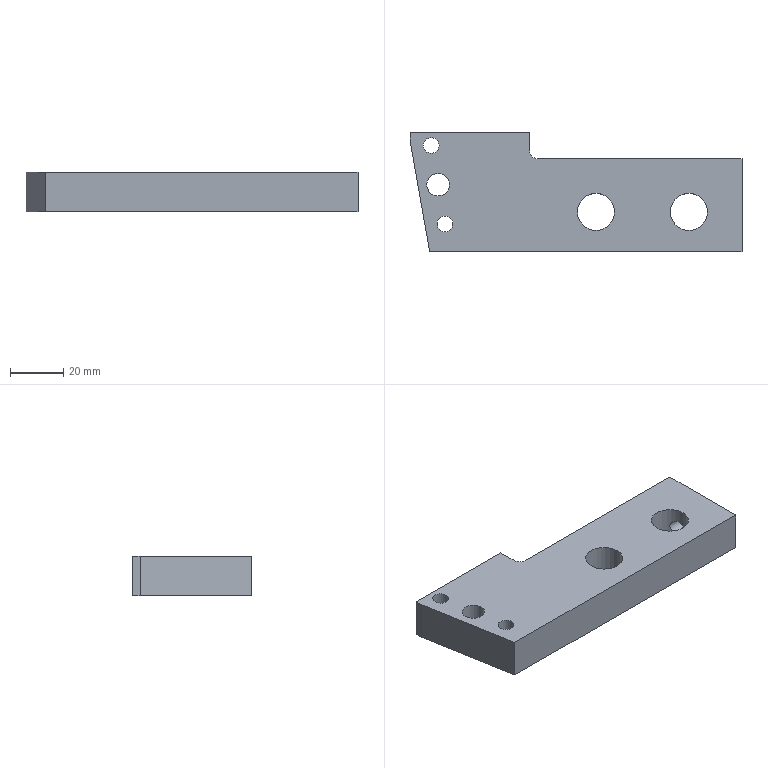Part | NX | features BREP 1 | 1 solid | 19 faces | box 125 x 45 x 15 mm | volume 63182 mm3 | plane 9 | cylinder 8 | cone 2 | commonest cylinder face diameters 6 x3 5 x2 14 x2 8.5 x1
STEP:
#1=CARTESIAN_POINT('',(62.5,-5.,-2.5));
#2=VERTEX_POINT('',#1);
#3=CARTESIAN_POINT('',(62.5,-5.,0.));
#4=DIRECTION('',(1.,0.,0.));
#5=DIRECTION('',(0.,0.,-1.));
#6=AXIS2_PLACEMENT_3D('',#3,#4,#5);
#7=CIRCLE('',#6,2.5);
#8=EDGE_CURVE('',#2,#2,#7,.T.);
#9=ORIENTED_EDGE('',*,*,#8,.F.);
#10=EDGE_LOOP('',(#9));
#11=FACE_BOUND('',#10,.T.);
#12=CARTESIAN_POINT('',(62.5,-22.5,-7.5));
#13=VERTEX_POINT('',#12);
#14=CARTESIAN_POINT('',(62.5,12.5,-7.5));
#15=VERTEX_POINT('',#14);
#16=CARTESIAN_POINT('',(62.5,-22.5,-7.5));
#17=DIRECTION('',(0.,1.,0.));
#18=VECTOR('',#17,1000.);
#19=LINE('',#16,#18);
#20=EDGE_CURVE('',#13,#15,#19,.T.);
#21=ORIENTED_EDGE('',*,*,#20,.T.);
#22=CARTESIAN_POINT('',(62.5,12.5,7.5));
#23=VERTEX_POINT('',#22);
#24=CARTESIAN_POINT('',(62.5,12.5,-88.123));
#25=DIRECTION('',(0.,0.,1.));
#26=VECTOR('',#25,1000.);
#27=LINE('',#24,#26);
#28=EDGE_CURVE('',#15,#23,#27,.T.);
#29=ORIENTED_EDGE('',*,*,#28,.T.);
#30=CARTESIAN_POINT('',(62.5,-22.5,7.5));
#31=VERTEX_POINT('',#30);
#32=CARTESIAN_POINT('',(62.5,-22.5,7.5));
#33=DIRECTION('',(0.,1.,0.));
#34=VECTOR('',#33,1000.);
#35=LINE('',#32,#34);
#36=EDGE_CURVE('',#31,#23,#35,.T.);
#37=ORIENTED_EDGE('',*,*,#36,.F.);
#38=CARTESIAN_POINT('',(62.5,-22.5,7.5));
#39=DIRECTION('',(0.,0.,-1.));
#40=VECTOR('',#39,1000.);
#41=LINE('',#38,#40);
#42=EDGE_CURVE('',#31,#13,#41,.T.);
#43=ORIENTED_EDGE('',*,*,#42,.T.);
#44=EDGE_LOOP('',(#21,#29,#37,#43));
#45=FACE_BOUND('',#44,.T.);
#46=CARTESIAN_POINT('',(62.5,-22.5,7.5));
#47=DIRECTION('',(-1.,0.,0.));
#48=DIRECTION('',(0.,0.,-1.));
#49=AXIS2_PLACEMENT_3D('',#46,#47,#48);
#50=PLANE('',#49);
#51=ADVANCED_FACE('',(#11,#45),#50,.F.);
#52=CARTESIAN_POINT('',(-17.5,22.5,7.5));
#53=VERTEX_POINT('',#52);
#54=CARTESIAN_POINT('',(-62.5,22.5,7.5));
#55=VERTEX_POINT('',#54);
#56=CARTESIAN_POINT('',(-62.5,22.5,7.5));
#57=DIRECTION('',(-1.,0.,0.));
#58=VECTOR('',#57,1000.);
#59=LINE('',#56,#58);
#60=EDGE_CURVE('',#53,#55,#59,.T.);
#61=ORIENTED_EDGE('',*,*,#60,.F.);
#62=CARTESIAN_POINT('',(-17.5,22.5,-7.5));
#63=VERTEX_POINT('',#62);
#64=CARTESIAN_POINT('',(-17.5,22.5,-88.123));
#65=DIRECTION('',(0.,0.,1.));
#66=VECTOR('',#65,1000.);
#67=LINE('',#64,#66);
#68=EDGE_CURVE('',#63,#53,#67,.T.);
#69=ORIENTED_EDGE('',*,*,#68,.F.);
#70=CARTESIAN_POINT('',(-62.5,22.5,-7.5));
#71=VERTEX_POINT('',#70);
#72=CARTESIAN_POINT('',(-62.5,22.5,-7.5));
#73=DIRECTION('',(-1.,0.,0.));
#74=VECTOR('',#73,1000.);
#75=LINE('',#72,#74);
#76=EDGE_CURVE('',#63,#71,#75,.T.);
#77=ORIENTED_EDGE('',*,*,#76,.T.);
#78=CARTESIAN_POINT('',(-62.5,22.5,7.5));
#79=DIRECTION('',(0.,0.,-1.));
#80=VECTOR('',#79,1000.);
#81=LINE('',#78,#80);
#82=EDGE_CURVE('',#55,#71,#81,.T.);
#83=ORIENTED_EDGE('',*,*,#82,.F.);
#84=EDGE_LOOP('',(#61,#69,#77,#83));
#85=FACE_BOUND('',#84,.T.);
#86=CARTESIAN_POINT('',(-62.5,22.5,7.5));
#87=DIRECTION('',(0.,-1.,0.));
#88=DIRECTION('',(0.,0.,1.));
#89=AXIS2_PLACEMENT_3D('',#86,#87,#88);
#90=PLANE('',#89);
#91=ADVANCED_FACE('',(#85),#90,.F.);
#92=CARTESIAN_POINT('',(-62.5,19.5,-7.5));
#93=VERTEX_POINT('',#92);
#94=CARTESIAN_POINT('',(-62.5,-22.5,-7.5));
#95=DIRECTION('',(0.,-1.,0.));
#96=VECTOR('',#95,1000.);
#97=LINE('',#94,#96);
#98=EDGE_CURVE('',#71,#93,#97,.T.);
#99=ORIENTED_EDGE('',*,*,#98,.T.);
#100=CARTESIAN_POINT('',(-62.5,19.5,7.5));
#101=VERTEX_POINT('',#100);
#102=CARTESIAN_POINT('',(-62.5,19.5,-50.148));
#103=DIRECTION('',(0.,0.,1.));
#104=VECTOR('',#103,1000.);
#105=LINE('',#102,#104);
#106=EDGE_CURVE('',#93,#101,#105,.T.);
#107=ORIENTED_EDGE('',*,*,#106,.T.);
#108=CARTESIAN_POINT('',(-62.5,-22.5,7.5));
#109=DIRECTION('',(0.,-1.,0.));
#110=VECTOR('',#109,1000.);
#111=LINE('',#108,#110);
#112=EDGE_CURVE('',#55,#101,#111,.T.);
#113=ORIENTED_EDGE('',*,*,#112,.F.);
#114=ORIENTED_EDGE('',*,*,#82,.T.);
#115=EDGE_LOOP('',(#99,#107,#113,#114));
#116=FACE_BOUND('',#115,.T.);
#117=CARTESIAN_POINT('',(-62.5,-22.5,7.5));
#118=DIRECTION('',(1.,0.,0.));
#119=DIRECTION('',(0.,0.,1.));
#120=AXIS2_PLACEMENT_3D('',#117,#118,#119);
#121=PLANE('',#120);
#122=ADVANCED_FACE('',(#116),#121,.F.);
#123=CARTESIAN_POINT('',(-55.094,-22.5,7.5));
#124=VERTEX_POINT('',#123);
#125=CARTESIAN_POINT('',(-62.5,-22.5,7.5));
#126=DIRECTION('',(1.,0.,0.));
#127=VECTOR('',#126,1000.);
#128=LINE('',#125,#127);
#129=EDGE_CURVE('',#124,#31,#128,.T.);
#130=ORIENTED_EDGE('',*,*,#129,.F.);
#131=CARTESIAN_POINT('',(-55.094,-22.5,-7.5));
#132=VERTEX_POINT('',#131);
#133=CARTESIAN_POINT('',(-55.094,-22.5,-50.148));
#134=DIRECTION('',(0.,0.,1.));
#135=VECTOR('',#134,1000.);
#136=LINE('',#133,#135);
#137=EDGE_CURVE('',#132,#124,#136,.T.);
#138=ORIENTED_EDGE('',*,*,#137,.F.);
#139=CARTESIAN_POINT('',(-62.5,-22.5,-7.5));
#140=DIRECTION('',(1.,0.,0.));
#141=VECTOR('',#140,1000.);
#142=LINE('',#139,#141);
#143=EDGE_CURVE('',#132,#13,#142,.T.);
#144=ORIENTED_EDGE('',*,*,#143,.T.);
#145=ORIENTED_EDGE('',*,*,#42,.F.);
#146=EDGE_LOOP('',(#130,#138,#144,#145));
#147=FACE_BOUND('',#146,.T.);
#148=CARTESIAN_POINT('',(-62.5,-22.5,7.5));
#149=DIRECTION('',(0.,1.,0.));
#150=DIRECTION('',(0.,0.,-1.));
#151=AXIS2_PLACEMENT_3D('',#148,#149,#150);
#152=PLANE('',#151);
#153=ADVANCED_FACE('',(#147),#152,.F.);
#154=CARTESIAN_POINT('',(49.5,-7.5,7.5));
#155=VERTEX_POINT('',#154);
#156=CARTESIAN_POINT('',(42.5,-7.5,7.5));
#157=DIRECTION('',(0.,0.,1.));
#158=DIRECTION('',(1.,0.,0.));
#159=AXIS2_PLACEMENT_3D('',#156,#157,#158);
#160=CIRCLE('',#159,7.);
#161=EDGE_CURVE('',#155,#155,#160,.T.);
#162=ORIENTED_EDGE('',*,*,#161,.F.);
#163=EDGE_LOOP('',(#162));
#164=FACE_BOUND('',#163,.T.);
#165=CARTESIAN_POINT('',(14.5,-7.5,7.5));
#166=VERTEX_POINT('',#165);
#167=CARTESIAN_POINT('',(7.5,-7.5,7.5));
#168=DIRECTION('',(0.,0.,1.));
#169=DIRECTION('',(1.,0.,0.));
#170=AXIS2_PLACEMENT_3D('',#167,#168,#169);
#171=CIRCLE('',#170,7.);
#172=EDGE_CURVE('',#166,#166,#171,.T.);
#173=ORIENTED_EDGE('',*,*,#172,.F.);
#174=EDGE_LOOP('',(#173));
#175=FACE_BOUND('',#174,.T.);
#176=CARTESIAN_POINT('',(-47.677,2.728,7.5));
#177=VERTEX_POINT('',#176);
#178=CARTESIAN_POINT('',(-51.927,2.728,7.5));
#179=DIRECTION('',(0.,0.,1.));
#180=DIRECTION('',(1.,0.,0.));
#181=AXIS2_PLACEMENT_3D('',#178,#179,#180);
#182=CIRCLE('',#181,4.25);
#183=EDGE_CURVE('',#177,#177,#182,.T.);
#184=ORIENTED_EDGE('',*,*,#183,.F.);
#185=EDGE_LOOP('',(#184));
#186=FACE_BOUND('',#185,.T.);
#187=CARTESIAN_POINT('',(-51.532,17.5,7.5));
#188=VERTEX_POINT('',#187);
#189=CARTESIAN_POINT('',(-54.532,17.5,7.5));
#190=DIRECTION('',(0.,0.,1.));
#191=DIRECTION('',(1.,0.,0.));
#192=AXIS2_PLACEMENT_3D('',#189,#190,#191);
#193=CIRCLE('',#192,3.);
#194=EDGE_CURVE('',#188,#188,#193,.T.);
#195=ORIENTED_EDGE('',*,*,#194,.F.);
#196=EDGE_LOOP('',(#195));
#197=FACE_BOUND('',#196,.T.);
#198=CARTESIAN_POINT('',(-46.322,-12.044,7.5));
#199=VERTEX_POINT('',#198);
#200=CARTESIAN_POINT('',(-49.322,-12.044,7.5));
#201=DIRECTION('',(0.,0.,1.));
#202=DIRECTION('',(1.,0.,0.));
#203=AXIS2_PLACEMENT_3D('',#200,#201,#202);
#204=CIRCLE('',#203,3.);
#205=EDGE_CURVE('',#199,#199,#204,.T.);
#206=ORIENTED_EDGE('',*,*,#205,.F.);
#207=EDGE_LOOP('',(#206));
#208=FACE_BOUND('',#207,.T.);
#209=CARTESIAN_POINT('',(-14.5,12.5,7.5));
#210=VERTEX_POINT('',#209);
#211=CARTESIAN_POINT('',(62.5,12.5,7.5));
#212=DIRECTION('',(1.,0.,0.));
#213=VECTOR('',#212,1000.);
#214=LINE('',#211,#213);
#215=EDGE_CURVE('',#210,#23,#214,.T.);
#216=ORIENTED_EDGE('',*,*,#215,.F.);
#217=CARTESIAN_POINT('',(-17.5,15.5,7.5));
#218=VERTEX_POINT('',#217);
#219=CARTESIAN_POINT('',(-14.5,15.5,7.5));
#220=DIRECTION('',(0.,0.,-1.));
#221=DIRECTION('',(-1.,0.,0.));
#222=AXIS2_PLACEMENT_3D('',#219,#220,#221);
#223=CIRCLE('',#222,3.);
#224=EDGE_CURVE('',#210,#218,#223,.T.);
#225=ORIENTED_EDGE('',*,*,#224,.T.);
#226=CARTESIAN_POINT('',(-17.5,12.5,7.5));
#227=DIRECTION('',(0.,-1.,0.));
#228=VECTOR('',#227,1000.);
#229=LINE('',#226,#228);
#230=EDGE_CURVE('',#53,#218,#229,.T.);
#231=ORIENTED_EDGE('',*,*,#230,.F.);
#232=ORIENTED_EDGE('',*,*,#60,.T.);
#233=ORIENTED_EDGE('',*,*,#112,.T.);
#234=CARTESIAN_POINT('',(-62.5,19.5,7.5));
#235=DIRECTION('',(-0.1736,0.9848,0.));
#236=VECTOR('',#235,1000.);
#237=LINE('',#234,#236);
#238=EDGE_CURVE('',#124,#101,#237,.T.);
#239=ORIENTED_EDGE('',*,*,#238,.F.);
#240=ORIENTED_EDGE('',*,*,#129,.T.);
#241=ORIENTED_EDGE('',*,*,#36,.T.);
#242=EDGE_LOOP('',(#216,#225,#231,#232,#233,#239,#240,#241));
#243=FACE_BOUND('',#242,.T.);
#244=CARTESIAN_POINT('',(0.,0.,7.5));
#245=DIRECTION('',(0.,0.,-1.));
#246=DIRECTION('',(1.,0.,0.));
#247=AXIS2_PLACEMENT_3D('',#244,#245,#246);
#248=PLANE('',#247);
#249=ADVANCED_FACE('',(#164,#175,#186,#197,#208,#243),#248,.F.);
#250=CARTESIAN_POINT('',(49.5,-7.5,-7.5));
#251=VERTEX_POINT('',#250);
#252=CARTESIAN_POINT('',(42.5,-7.5,-7.5));
#253=DIRECTION('',(0.,0.,1.));
#254=DIRECTION('',(1.,0.,0.));
#255=AXIS2_PLACEMENT_3D('',#252,#253,#254);
#256=CIRCLE('',#255,7.);
#257=EDGE_CURVE('',#251,#251,#256,.T.);
#258=ORIENTED_EDGE('',*,*,#257,.T.);
#259=EDGE_LOOP('',(#258));
#260=FACE_BOUND('',#259,.T.);
#261=CARTESIAN_POINT('',(14.5,-7.5,-7.5));
#262=VERTEX_POINT('',#261);
#263=CARTESIAN_POINT('',(7.5,-7.5,-7.5));
#264=DIRECTION('',(0.,0.,1.));
#265=DIRECTION('',(1.,0.,0.));
#266=AXIS2_PLACEMENT_3D('',#263,#264,#265);
#267=CIRCLE('',#266,7.);
#268=EDGE_CURVE('',#262,#262,#267,.T.);
#269=ORIENTED_EDGE('',*,*,#268,.T.);
#270=EDGE_LOOP('',(#269));
#271=FACE_BOUND('',#270,.T.);
#272=CARTESIAN_POINT('',(-17.5,15.5,-7.5));
#273=VERTEX_POINT('',#272);
#274=CARTESIAN_POINT('',(-17.5,12.5,-7.5));
#275=DIRECTION('',(0.,-1.,0.));
#276=VECTOR('',#275,1000.);
#277=LINE('',#274,#276);
#278=EDGE_CURVE('',#63,#273,#277,.T.);
#279=ORIENTED_EDGE('',*,*,#278,.T.);
#280=CARTESIAN_POINT('',(-14.5,12.5,-7.5));
#281=VERTEX_POINT('',#280);
#282=CARTESIAN_POINT('',(-14.5,15.5,-7.5));
#283=DIRECTION('',(0.,0.,1.));
#284=DIRECTION('',(-1.,0.,0.));
#285=AXIS2_PLACEMENT_3D('',#282,#283,#284);
#286=CIRCLE('',#285,3.);
#287=EDGE_CURVE('',#273,#281,#286,.T.);
#288=ORIENTED_EDGE('',*,*,#287,.T.);
#289=CARTESIAN_POINT('',(62.5,12.5,-7.5));
#290=DIRECTION('',(1.,0.,0.));
#291=VECTOR('',#290,1000.);
#292=LINE('',#289,#291);
#293=EDGE_CURVE('',#281,#15,#292,.T.);
#294=ORIENTED_EDGE('',*,*,#293,.T.);
#295=ORIENTED_EDGE('',*,*,#20,.F.);
#296=ORIENTED_EDGE('',*,*,#143,.F.);
#297=CARTESIAN_POINT('',(-62.5,19.5,-7.5));
#298=DIRECTION('',(-0.1736,0.9848,0.));
#299=VECTOR('',#298,1000.);
#300=LINE('',#297,#299);
#301=EDGE_CURVE('',#132,#93,#300,.T.);
#302=ORIENTED_EDGE('',*,*,#301,.T.);
#303=ORIENTED_EDGE('',*,*,#98,.F.);
#304=ORIENTED_EDGE('',*,*,#76,.F.);
#305=EDGE_LOOP('',(#279,#288,#294,#295,#296,#302,#303,#304));
#306=FACE_BOUND('',#305,.T.);
#307=CARTESIAN_POINT('',(-47.677,2.728,-7.5));
#308=VERTEX_POINT('',#307);
#309=CARTESIAN_POINT('',(-51.927,2.728,-7.5));
#310=DIRECTION('',(0.,0.,1.));
#311=DIRECTION('',(1.,0.,0.));
#312=AXIS2_PLACEMENT_3D('',#309,#310,#311);
#313=CIRCLE('',#312,4.25);
#314=EDGE_CURVE('',#308,#308,#313,.T.);
#315=ORIENTED_EDGE('',*,*,#314,.T.);
#316=EDGE_LOOP('',(#315));
#317=FACE_BOUND('',#316,.T.);
#318=CARTESIAN_POINT('',(-51.532,17.5,-7.5));
#319=VERTEX_POINT('',#318);
#320=CARTESIAN_POINT('',(-54.532,17.5,-7.5));
#321=DIRECTION('',(0.,0.,1.));
#322=DIRECTION('',(1.,0.,0.));
#323=AXIS2_PLACEMENT_3D('',#320,#321,#322);
#324=CIRCLE('',#323,3.);
#325=EDGE_CURVE('',#319,#319,#324,.T.);
#326=ORIENTED_EDGE('',*,*,#325,.T.);
#327=EDGE_LOOP('',(#326));
#328=FACE_BOUND('',#327,.T.);
#329=CARTESIAN_POINT('',(-46.322,-12.044,-7.5));
#330=VERTEX_POINT('',#329);
#331=CARTESIAN_POINT('',(-49.322,-12.044,-7.5));
#332=DIRECTION('',(0.,0.,1.));
#333=DIRECTION('',(1.,0.,0.));
#334=AXIS2_PLACEMENT_3D('',#331,#332,#333);
#335=CIRCLE('',#334,3.);
#336=EDGE_CURVE('',#330,#330,#335,.T.);
#337=ORIENTED_EDGE('',*,*,#336,.T.);
#338=EDGE_LOOP('',(#337));
#339=FACE_BOUND('',#338,.T.);
#340=CARTESIAN_POINT('',(0.,0.,-7.5));
#341=DIRECTION('',(0.,0.,-1.));
#342=DIRECTION('',(1.,0.,0.));
#343=AXIS2_PLACEMENT_3D('',#340,#341,#342);
#344=PLANE('',#343);
#345=ADVANCED_FACE('',(#260,#271,#306,#317,#328,#339),#344,.T.);
#346=ORIENTED_EDGE('',*,*,#137,.T.);
#347=ORIENTED_EDGE('',*,*,#238,.T.);
#348=ORIENTED_EDGE('',*,*,#106,.F.);
#349=ORIENTED_EDGE('',*,*,#301,.F.);
#350=EDGE_LOOP('',(#346,#347,#348,#349));
#351=FACE_BOUND('',#350,.T.);
#352=CARTESIAN_POINT('',(-62.5,19.5,-50.148));
#353=DIRECTION('',(0.9848,0.1736,0.));
#354=DIRECTION('',(0.1736,-0.9848,0.));
#355=AXIS2_PLACEMENT_3D('',#352,#353,#354);
#356=PLANE('',#355);
#357=ADVANCED_FACE('',(#351),#356,.F.);
#358=ORIENTED_EDGE('',*,*,#336,.F.);
#359=EDGE_LOOP('',(#358));
#360=FACE_BOUND('',#359,.T.);
#361=ORIENTED_EDGE('',*,*,#205,.T.);
#362=EDGE_LOOP('',(#361));
#363=FACE_BOUND('',#362,.T.);
#364=CARTESIAN_POINT('',(-49.322,-12.044,7.5));
#365=DIRECTION('',(0.,0.,1.));
#366=DIRECTION('',(-1.,0.,0.));
#367=AXIS2_PLACEMENT_3D('',#364,#365,#366);
#368=CYLINDRICAL_SURFACE('',#367,3.);
#369=ADVANCED_FACE('',(#360,#363),#368,.F.);
#370=ORIENTED_EDGE('',*,*,#325,.F.);
#371=EDGE_LOOP('',(#370));
#372=FACE_BOUND('',#371,.T.);
#373=ORIENTED_EDGE('',*,*,#194,.T.);
#374=EDGE_LOOP('',(#373));
#375=FACE_BOUND('',#374,.T.);
#376=CARTESIAN_POINT('',(-54.532,17.5,7.5));
#377=DIRECTION('',(0.,0.,1.));
#378=DIRECTION('',(-1.,0.,0.));
#379=AXIS2_PLACEMENT_3D('',#376,#377,#378);
#380=CYLINDRICAL_SURFACE('',#379,3.);
#381=ADVANCED_FACE('',(#372,#375),#380,.F.);
#382=ORIENTED_EDGE('',*,*,#314,.F.);
#383=EDGE_LOOP('',(#382));
#384=FACE_BOUND('',#383,.T.);
#385=ORIENTED_EDGE('',*,*,#183,.T.);
#386=EDGE_LOOP('',(#385));
#387=FACE_BOUND('',#386,.T.);
#388=CARTESIAN_POINT('',(-51.927,2.728,7.5));
#389=DIRECTION('',(0.,0.,1.));
#390=DIRECTION('',(-1.,0.,0.));
#391=AXIS2_PLACEMENT_3D('',#388,#389,#390);
#392=CYLINDRICAL_SURFACE('',#391,4.25);
#393=ADVANCED_FACE('',(#384,#387),#392,.F.);
#394=ORIENTED_EDGE('',*,*,#230,.T.);
#395=CARTESIAN_POINT('',(-17.5,15.5,-7.5));
#396=DIRECTION('',(0.,0.,-1.));
#397=VECTOR('',#396,1000.);
#398=LINE('',#395,#397);
#399=EDGE_CURVE('',#218,#273,#398,.T.);
#400=ORIENTED_EDGE('',*,*,#399,.T.);
#401=ORIENTED_EDGE('',*,*,#278,.F.);
#402=ORIENTED_EDGE('',*,*,#68,.T.);
#403=EDGE_LOOP('',(#394,#400,#401,#402));
#404=FACE_BOUND('',#403,.T.);
#405=CARTESIAN_POINT('',(-17.5,12.5,-88.123));
#406=DIRECTION('',(-1.,0.,0.));
#407=DIRECTION('',(0.,0.,-1.));
#408=AXIS2_PLACEMENT_3D('',#405,#406,#407);
#409=PLANE('',#408);
#410=ADVANCED_FACE('',(#404),#409,.F.);
#411=CARTESIAN_POINT('',(17.5,12.5,2.5));
#412=VERTEX_POINT('',#411);
#413=CARTESIAN_POINT('',(17.5,12.5,0.));
#414=DIRECTION('',(0.,1.,0.));
#415=DIRECTION('',(0.,0.,1.));
#416=AXIS2_PLACEMENT_3D('',#413,#414,#415);
#417=CIRCLE('',#416,2.5);
#418=EDGE_CURVE('',#412,#412,#417,.T.);
#419=ORIENTED_EDGE('',*,*,#418,.F.);
#420=EDGE_LOOP('',(#419));
#421=FACE_BOUND('',#420,.T.);
#422=ORIENTED_EDGE('',*,*,#293,.F.);
#423=CARTESIAN_POINT('',(-14.5,12.5,7.5));
#424=DIRECTION('',(0.,0.,1.));
#425=VECTOR('',#424,1000.);
#426=LINE('',#423,#425);
#427=EDGE_CURVE('',#281,#210,#426,.T.);
#428=ORIENTED_EDGE('',*,*,#427,.T.);
#429=ORIENTED_EDGE('',*,*,#215,.T.);
#430=ORIENTED_EDGE('',*,*,#28,.F.);
#431=EDGE_LOOP('',(#422,#428,#429,#430));
#432=FACE_BOUND('',#431,.T.);
#433=CARTESIAN_POINT('',(62.5,12.5,-88.123));
#434=DIRECTION('',(0.,-1.,0.));
#435=DIRECTION('',(-1.,0.,0.));
#436=AXIS2_PLACEMENT_3D('',#433,#434,#435);
#437=PLANE('',#436);
#438=ADVANCED_FACE('',(#421,#432),#437,.F.);
#439=ORIENTED_EDGE('',*,*,#268,.F.);
#440=EDGE_LOOP('',(#439));
#441=FACE_BOUND('',#440,.T.);
#442=ORIENTED_EDGE('',*,*,#172,.T.);
#443=EDGE_LOOP('',(#442));
#444=FACE_BOUND('',#443,.T.);
#445=CARTESIAN_POINT('',(7.5,-7.5,7.5));
#446=DIRECTION('',(0.,0.,1.));
#447=DIRECTION('',(-1.,0.,0.));
#448=AXIS2_PLACEMENT_3D('',#445,#446,#447);
#449=CYLINDRICAL_SURFACE('',#448,7.);
#450=ADVANCED_FACE('',(#441,#444),#449,.F.);
#451=CARTESIAN_POINT('',(47.5,-2.601,-0.7035));
#452=VERTEX_POINT('',#451);
#453=CARTESIAN_POINT('',(47.5,-2.601,0.7035));
#454=VERTEX_POINT('',#453);
#455=CARTESIAN_POINT('',(47.5,-2.601,-0.7035));
#456=CARTESIAN_POINT('',(47.45,-2.55,-0.2345));
#457=CARTESIAN_POINT('',(47.45,-2.55,0.2345));
#458=CARTESIAN_POINT('',(47.5,-2.601,0.7035));
#459=B_SPLINE_CURVE_WITH_KNOTS('',3,(#455,#456,#457,#458),.UNSPECIFIED.,.F.,.F.,(4,4),(0.,0.001407),.UNSPECIFIED.);
#460=EDGE_CURVE('',#452,#454,#459,.T.);
#461=ORIENTED_EDGE('',*,*,#460,.T.);
#462=CARTESIAN_POINT('',(47.5,-2.601,0.7035));
#463=CARTESIAN_POINT('',(47.669,-2.774,1.292));
#464=CARTESIAN_POINT('',(48.313,-3.475,2.198));
#465=CARTESIAN_POINT('',(49.199,-5.161,2.716));
#466=CARTESIAN_POINT('',(49.528,-6.996,1.898));
#467=CARTESIAN_POINT('',(49.486,-7.75,0.005277));
#468=CARTESIAN_POINT('',(49.528,-7.006,-1.885));
#469=CARTESIAN_POINT('',(49.205,-5.176,-2.717));
#470=CARTESIAN_POINT('',(48.312,-3.472,-2.199));
#471=CARTESIAN_POINT('',(47.669,-2.774,-1.293));
#472=CARTESIAN_POINT('',(47.5,-2.601,-0.7035));
#473=B_SPLINE_CURVE_WITH_KNOTS('',3,(#462,#463,#464,#465,#466,#467,#468,#469,#470,#471,#472),.UNSPECIFIED.,.F.,.F.,(4,1,1,1,1,1,1,1,4),(0.,0.001875,0.003749,0.005624,0.007499,0.009373,0.01125,0.01312,0.015),.UNSPECIFIED.);
#474=EDGE_CURVE('',#454,#452,#473,.T.);
#475=ORIENTED_EDGE('',*,*,#474,.T.);
#476=EDGE_LOOP('',(#461,#475));
#477=FACE_BOUND('',#476,.T.);
#478=ORIENTED_EDGE('',*,*,#257,.F.);
#479=EDGE_LOOP('',(#478));
#480=FACE_BOUND('',#479,.T.);
#481=ORIENTED_EDGE('',*,*,#161,.T.);
#482=EDGE_LOOP('',(#481));
#483=FACE_BOUND('',#482,.T.);
#484=CARTESIAN_POINT('',(42.5,-7.5,7.5));
#485=DIRECTION('',(0.,0.,1.));
#486=DIRECTION('',(-1.,0.,0.));
#487=AXIS2_PLACEMENT_3D('',#484,#485,#486);
#488=CYLINDRICAL_SURFACE('',#487,7.);
#489=ADVANCED_FACE('',(#477,#480,#483),#488,.F.);
#490=ORIENTED_EDGE('',*,*,#8,.T.);
#491=EDGE_LOOP('',(#490));
#492=FACE_BOUND('',#491,.T.);
#493=CARTESIAN_POINT('',(47.5,-5.,0.));
#494=DIRECTION('',(1.,0.,0.));
#495=DIRECTION('',(0.,0.,-1.));
#496=AXIS2_PLACEMENT_3D('',#493,#494,#495);
#497=CIRCLE('',#496,2.5);
#498=EDGE_CURVE('',#452,#454,#497,.T.);
#499=ORIENTED_EDGE('',*,*,#498,.F.);
#500=ORIENTED_EDGE('',*,*,#474,.F.);
#501=EDGE_LOOP('',(#499,#500));
#502=FACE_BOUND('',#501,.T.);
#503=CARTESIAN_POINT('',(62.5,-5.,0.));
#504=DIRECTION('',(1.,0.,0.));
#505=DIRECTION('',(0.,0.,1.));
#506=AXIS2_PLACEMENT_3D('',#503,#504,#505);
#507=CYLINDRICAL_SURFACE('',#506,2.5);
#508=ADVANCED_FACE('',(#492,#502),#507,.F.);
#509=ORIENTED_EDGE('',*,*,#498,.T.);
#510=ORIENTED_EDGE('',*,*,#460,.F.);
#511=EDGE_LOOP('',(#509,#510));
#512=FACE_BOUND('',#511,.T.);
#513=CARTESIAN_POINT('',(47.5,-5.,0.));
#514=DIRECTION('',(1.,0.,0.));
#515=DIRECTION('',(0.,0.,1.));
#516=AXIS2_PLACEMENT_3D('',#513,#514,#515);
#517=CONICAL_SURFACE('',#516,2.5,1.03);
#518=ADVANCED_FACE('',(#512),#517,.F.);
#519=CARTESIAN_POINT('',(17.5,-4.002,0.));
#520=VERTEX_POINT('',#519);
#521=VERTEX_LOOP('',#520);
#522=FACE_BOUND('',#521,.T.);
#523=CARTESIAN_POINT('',(17.5,-2.5,2.5));
#524=VERTEX_POINT('',#523);
#525=CARTESIAN_POINT('',(17.5,-2.5,0.));
#526=DIRECTION('',(0.,1.,0.));
#527=DIRECTION('',(0.,0.,1.));
#528=AXIS2_PLACEMENT_3D('',#525,#526,#527);
#529=CIRCLE('',#528,2.5);
#530=EDGE_CURVE('',#524,#524,#529,.T.);
#531=ORIENTED_EDGE('',*,*,#530,.T.);
#532=EDGE_LOOP('',(#531));
#533=FACE_BOUND('',#532,.T.);
#534=CARTESIAN_POINT('',(17.5,-2.5,0.));
#535=DIRECTION('',(0.,1.,0.));
#536=DIRECTION('',(0.,0.,-1.));
#537=AXIS2_PLACEMENT_3D('',#534,#535,#536);
#538=CONICAL_SURFACE('',#537,2.5,1.03);
#539=ADVANCED_FACE('',(#522,#533),#538,.F.);
#540=ORIENTED_EDGE('',*,*,#530,.F.);
#541=EDGE_LOOP('',(#540));
#542=FACE_BOUND('',#541,.T.);
#543=ORIENTED_EDGE('',*,*,#418,.T.);
#544=EDGE_LOOP('',(#543));
#545=FACE_BOUND('',#544,.T.);
#546=CARTESIAN_POINT('',(17.5,12.5,0.));
#547=DIRECTION('',(0.,1.,0.));
#548=DIRECTION('',(0.,0.,-1.));
#549=AXIS2_PLACEMENT_3D('',#546,#547,#548);
#550=CYLINDRICAL_SURFACE('',#549,2.5);
#551=ADVANCED_FACE('',(#542,#545),#550,.F.);
#552=ORIENTED_EDGE('',*,*,#287,.F.);
#553=ORIENTED_EDGE('',*,*,#399,.F.);
#554=ORIENTED_EDGE('',*,*,#224,.F.);
#555=ORIENTED_EDGE('',*,*,#427,.F.);
#556=EDGE_LOOP('',(#552,#553,#554,#555));
#557=FACE_BOUND('',#556,.T.);
#558=CARTESIAN_POINT('',(-14.5,15.5,-88.123));
#559=DIRECTION('',(0.,0.,-1.));
#560=DIRECTION('',(1.,0.,0.));
#561=AXIS2_PLACEMENT_3D('',#558,#559,#560);
#562=CYLINDRICAL_SURFACE('',#561,3.);
#563=ADVANCED_FACE('',(#557),#562,.F.);
#564=CLOSED_SHELL('',(#51,#91,#122,#153,#249,#345,#357,#369,#381,#393,#410,#438,#450,#489,#508,#518,#539,#551,#563));
#565=MANIFOLD_SOLID_BREP('',#564);
#566=(LENGTH_UNIT()NAMED_UNIT(*)SI_UNIT(.MILLI.,.METRE.));
#567=UNCERTAINTY_MEASURE_WITH_UNIT(LENGTH_MEASURE(0.0508),#566,'','');
#568=(NAMED_UNIT(*)PLANE_ANGLE_UNIT()SI_UNIT($,.RADIAN.));
#569=(NAMED_UNIT(*)SI_UNIT($,.STERADIAN.)SOLID_ANGLE_UNIT());
#570=(GEOMETRIC_REPRESENTATION_CONTEXT(3)GLOBAL_UNCERTAINTY_ASSIGNED_CONTEXT((#567))GLOBAL_UNIT_ASSIGNED_CONTEXT((#566,#568,#569))REPRESENTATION_CONTEXT('',''));
#571=ADVANCED_BREP_SHAPE_REPRESENTATION('',(#565),#570);